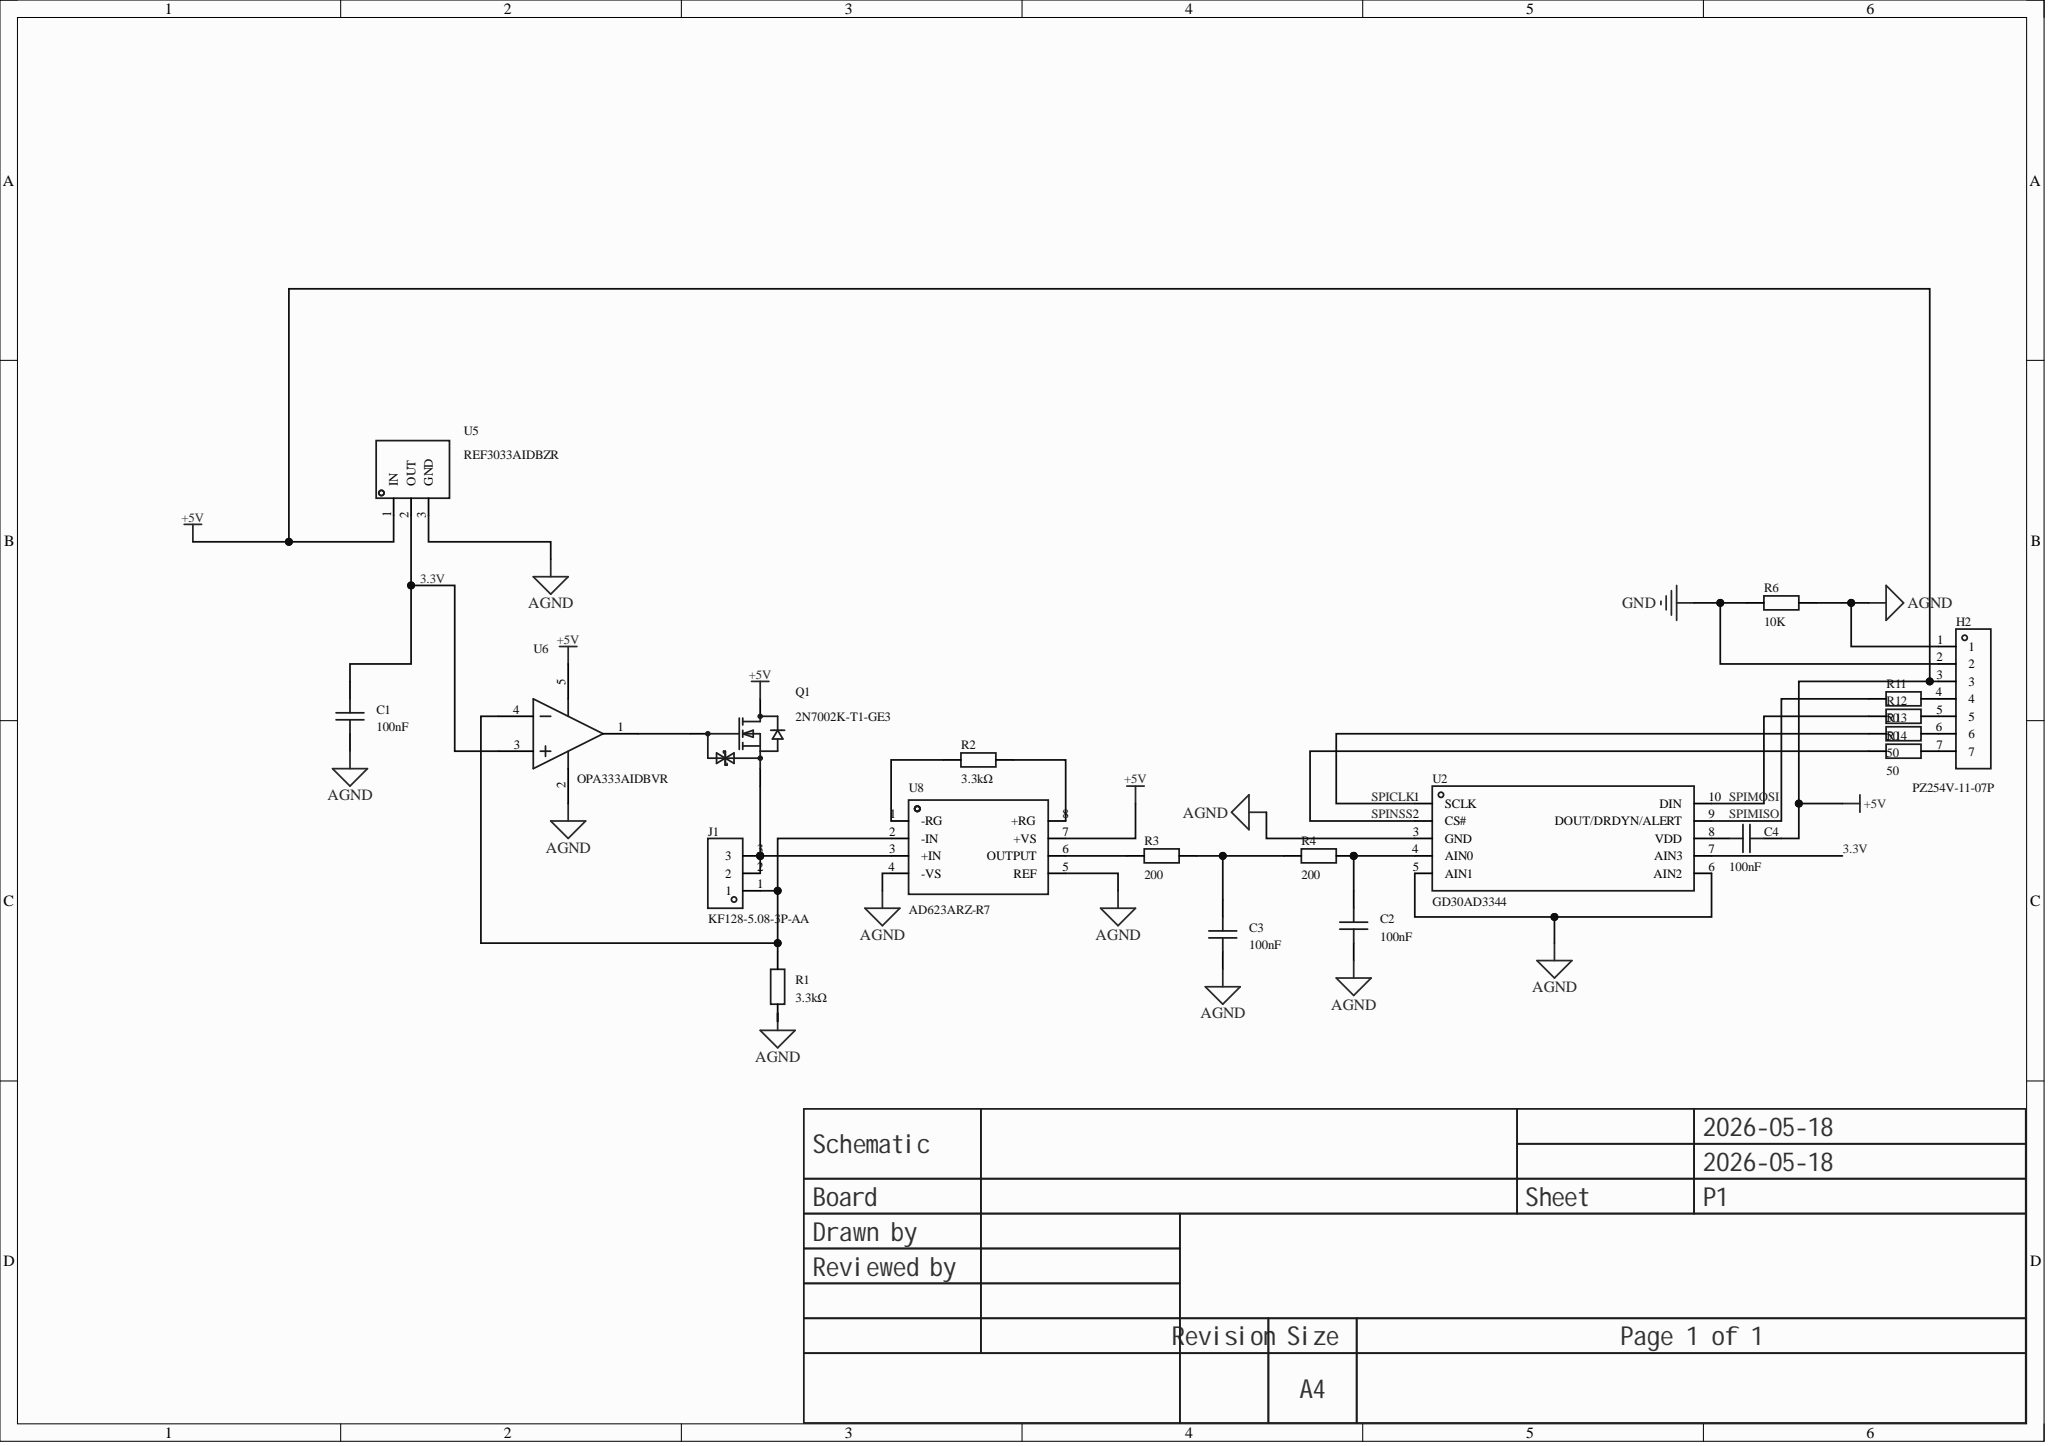Circuit board | Altium Designer | 20 parts | 21 nets
Bill of materials:
Comment,Description,Designator,Footprint,LibRef,Quantity
"100nF","","C1, C2, C3, C4","C0805","CAP_0805","4"
"PZ254V-11-07P","","H2","HDR-TH_7P-P2.54-V-M","PZ254V-11-07P","1"
"KF128-5.08-3P-AA","","J1","CONN-TH_3P-P5.08_KF128-5.08-3P","KF128-5.08-3P-AA","1"
"2N7002K-T1-GE3","","Q1","SOT-23-3_L2.9-W1.6-P1.90-LS2.8-BR","2N7002K-T1-GE3","1"
"3.3kΩ","","R1, R2","Res_1/4W","Res_AXIAL-1/4W","2"
"200","","R3, R4","Res_1/4W","Res_AXIAL-1/4W","2"
"10K","","R6","Res_1/4W","Res_AXIAL-1/4W","1"
"50","","R11, R12, R13, R14","R0805","Res_0805","4"
"GD30AD3344","","U2","MSOP-10_L3.0-W3.0-P0.50-LS5.0-BL","GD30AD3344","1"
"REF3033AIDBZR","","U5","SOT-23-3_L3.0-W1.7-P0.95-LS2.9-BR","REF3033AIDBZR","1"
"OPA333AIDBVR","","U6","SOT-23-5_L3.0-W1.7-P0.95-LS2.8-BR","OPA333AIDBVR","1"
"AD623ARZ-R7","","U8","SOIC-8_L5.0-W4.0-P1.27-LS6.0-BL","AD623ARZ-R7","1"
Netlist (Protel format):
[
C1
C0805
100nF



]
[
C2
C0805
100nF



]
[
C3
C0805
100nF



]
[
C4
C0805
100nF



]
[
H2
HDR-TH_7P-P2.54-V-M
PZ254V-11-07P



]
[
J1
CONN-TH_3P-P5.08_KF128-5.08-3P
KF128-5.08-3P-AA



]
[
Q1
SOT-23-3_L2.9-W1.6-P1.90-LS2.8-BR
2N7002K-T1-GE3



]
[
R1
Res_1/4W
3.3kΩ



]
[
R2
Res_1/4W
3.3kΩ



]
[
R3
Res_1/4W
200



]
[
R4
Res_1/4W
200



]
[
R6
Res_1/4W
10K



]
[
R11
R0805
50



]
[
R12
R0805
50



]
[
R13
R0805
50



]
[
R14
R0805
50



]
[
U2
MSOP-10_L3.0-W3.0-P0.50-LS5.0-BL
GD30AD3344



]
[
U5
SOT-23-3_L3.0-W1.7-P0.95-LS2.9-BR
REF3033AIDBZR



]
[
U6
SOT-23-5_L3.0-W1.7-P0.95-LS2.8-BR
OPA333AIDBVR



]
[
U8
SOIC-8_L5.0-W4.0-P1.27-LS6.0-BL
AD623ARZ-R7



]
(
SPINSS
R14-1
U2-2
)
(
SPIMOSI
R12-1
U2-10
)
(
SPIMISO
R11-1
U2-9
)
(
SPICLK
R13-1
U2-1
)
(
NetR3_1
R3-1
U8-6
)
(
NetR2_2
R2-2
U8-8
)
(
NetR2_1
R2-1
U8-1
)
(
NetQ1_1
Q1-1
U6-1
)
(
NetJ1_2
J1-2
J1-3
Q1-2
U8-3
)
(
NetJ1_1
J1-1
R1-2
U6-4
U8-2
)
(
NetH2_7
H2-7
R14-2
)
(
NetH2_6
H2-6
R13-2
)
(
NetH2_5
H2-5
R12-2
)
(
NetH2_4
H2-4
R11-2
)
(
NetC4_1
C4-1
U2-8
)
(
NetC3_2
C3-2
R3-2
R4-1
)
(
NetC2_2
C2-2
R4-2
U2-4
)
(
GND
H2-2
R6-1
)
(
AGND
C1-1
C2-1
C3-1
H2-1
R1-1
R6-2
U2-3
U2-5
U2-6
U5-3
U6-2
U8-4
U8-5
)
(
+5V
C4-2
H2-3
Q1-3
U5-1
U6-5
U8-7
)
(
3.3V
C1-2
U2-7
U5-2
U6-3
)